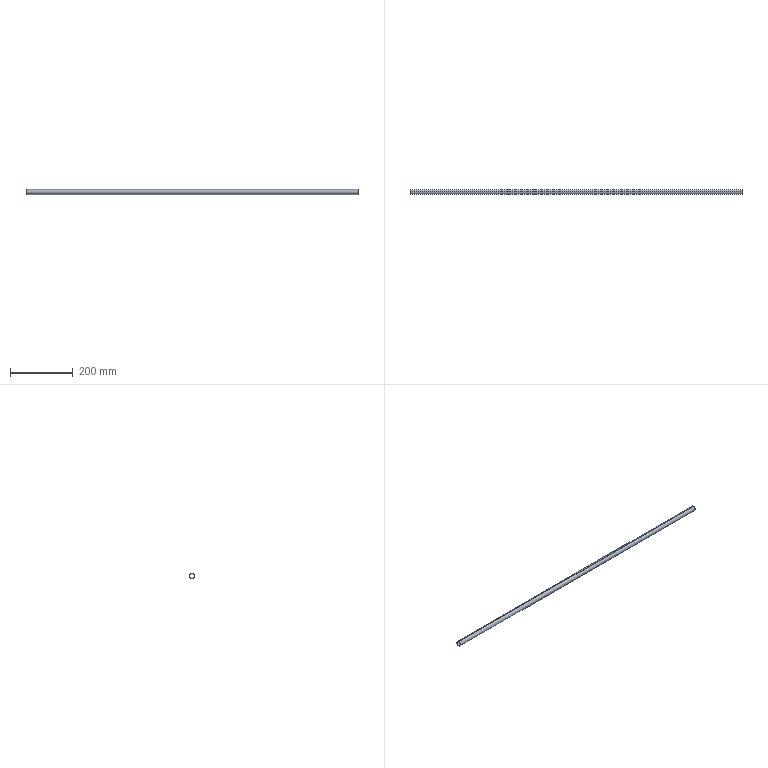Part | NX | features BREP 1 | 1 solid | 6 faces | box 1055 x 16 x 16 mm | volume 25686 mm3 | cylinder 4 | plane 2 | commonest cylinder face diameters 15 x2 16 x2
STEP:
#1=CARTESIAN_POINT('',(1055.,0.,7.5));
#2=VERTEX_POINT('',#1);
#3=CARTESIAN_POINT('',(1055.,0.,-7.5));
#4=VERTEX_POINT('',#3);
#5=CARTESIAN_POINT('',(1055.,0.,0.));
#6=DIRECTION('',(1.,0.,0.));
#7=DIRECTION('',(0.,0.,-1.));
#8=AXIS2_PLACEMENT_3D('',#5,#6,#7);
#9=CIRCLE('',#8,7.5);
#10=EDGE_CURVE('',#2,#4,#9,.T.);
#11=ORIENTED_EDGE('',*,*,#10,.T.);
#12=CARTESIAN_POINT('',(0.,0.,-7.5));
#13=VERTEX_POINT('',#12);
#14=CARTESIAN_POINT('',(1055.,0.,-7.5));
#15=DIRECTION('',(-1.,0.,0.));
#16=VECTOR('',#15,1000.);
#17=LINE('',#14,#16);
#18=EDGE_CURVE('',#4,#13,#17,.T.);
#19=ORIENTED_EDGE('',*,*,#18,.T.);
#20=CARTESIAN_POINT('',(0.,0.,7.5));
#21=VERTEX_POINT('',#20);
#22=CARTESIAN_POINT('',(0.,0.,0.));
#23=DIRECTION('',(1.,0.,0.));
#24=DIRECTION('',(0.,0.,-1.));
#25=AXIS2_PLACEMENT_3D('',#22,#23,#24);
#26=CIRCLE('',#25,7.5);
#27=EDGE_CURVE('',#21,#13,#26,.T.);
#28=ORIENTED_EDGE('',*,*,#27,.F.);
#29=CARTESIAN_POINT('',(1055.,0.,7.5));
#30=DIRECTION('',(-1.,0.,0.));
#31=VECTOR('',#30,1000.);
#32=LINE('',#29,#31);
#33=EDGE_CURVE('',#2,#21,#32,.T.);
#34=ORIENTED_EDGE('',*,*,#33,.F.);
#35=EDGE_LOOP('',(#11,#19,#28,#34));
#36=FACE_BOUND('',#35,.T.);
#37=CARTESIAN_POINT('',(1055.,0.,0.));
#38=DIRECTION('',(-1.,0.,0.));
#39=DIRECTION('',(0.,0.,-1.));
#40=AXIS2_PLACEMENT_3D('',#37,#38,#39);
#41=CYLINDRICAL_SURFACE('',#40,7.5);
#42=ADVANCED_FACE('',(#36),#41,.F.);
#43=CARTESIAN_POINT('',(1055.,0.,-8.));
#44=VERTEX_POINT('',#43);
#45=CARTESIAN_POINT('',(1055.,0.,8.));
#46=VERTEX_POINT('',#45);
#47=CARTESIAN_POINT('',(1055.,0.,0.));
#48=DIRECTION('',(1.,0.,0.));
#49=DIRECTION('',(0.,0.,-1.));
#50=AXIS2_PLACEMENT_3D('',#47,#48,#49);
#51=CIRCLE('',#50,8.);
#52=EDGE_CURVE('',#44,#46,#51,.T.);
#53=ORIENTED_EDGE('',*,*,#52,.F.);
#54=CARTESIAN_POINT('',(0.,0.,-8.));
#55=VERTEX_POINT('',#54);
#56=CARTESIAN_POINT('',(1055.,0.,-8.));
#57=DIRECTION('',(-1.,0.,0.));
#58=VECTOR('',#57,1000.);
#59=LINE('',#56,#58);
#60=EDGE_CURVE('',#44,#55,#59,.T.);
#61=ORIENTED_EDGE('',*,*,#60,.T.);
#62=CARTESIAN_POINT('',(0.,0.,8.));
#63=VERTEX_POINT('',#62);
#64=CARTESIAN_POINT('',(0.,0.,0.));
#65=DIRECTION('',(1.,0.,0.));
#66=DIRECTION('',(0.,0.,-1.));
#67=AXIS2_PLACEMENT_3D('',#64,#65,#66);
#68=CIRCLE('',#67,8.);
#69=EDGE_CURVE('',#55,#63,#68,.T.);
#70=ORIENTED_EDGE('',*,*,#69,.T.);
#71=CARTESIAN_POINT('',(1055.,0.,8.));
#72=DIRECTION('',(-1.,0.,0.));
#73=VECTOR('',#72,1000.);
#74=LINE('',#71,#73);
#75=EDGE_CURVE('',#46,#63,#74,.T.);
#76=ORIENTED_EDGE('',*,*,#75,.F.);
#77=EDGE_LOOP('',(#53,#61,#70,#76));
#78=FACE_BOUND('',#77,.T.);
#79=CARTESIAN_POINT('',(1055.,0.,0.));
#80=DIRECTION('',(-1.,0.,0.));
#81=DIRECTION('',(0.,0.,-1.));
#82=AXIS2_PLACEMENT_3D('',#79,#80,#81);
#83=CYLINDRICAL_SURFACE('',#82,8.);
#84=ADVANCED_FACE('',(#78),#83,.T.);
#85=CARTESIAN_POINT('',(1055.,0.,0.));
#86=DIRECTION('',(1.,0.,0.));
#87=DIRECTION('',(0.,0.,-1.));
#88=AXIS2_PLACEMENT_3D('',#85,#86,#87);
#89=CIRCLE('',#88,8.);
#90=EDGE_CURVE('',#46,#44,#89,.T.);
#91=ORIENTED_EDGE('',*,*,#90,.T.);
#92=ORIENTED_EDGE('',*,*,#52,.T.);
#93=EDGE_LOOP('',(#91,#92));
#94=FACE_BOUND('',#93,.T.);
#95=ORIENTED_EDGE('',*,*,#10,.F.);
#96=CARTESIAN_POINT('',(1055.,0.,0.));
#97=DIRECTION('',(1.,0.,0.));
#98=DIRECTION('',(0.,0.,-1.));
#99=AXIS2_PLACEMENT_3D('',#96,#97,#98);
#100=CIRCLE('',#99,7.5);
#101=EDGE_CURVE('',#4,#2,#100,.T.);
#102=ORIENTED_EDGE('',*,*,#101,.F.);
#103=EDGE_LOOP('',(#95,#102));
#104=FACE_BOUND('',#103,.T.);
#105=CARTESIAN_POINT('',(1055.,0.,0.));
#106=DIRECTION('',(1.,0.,0.));
#107=DIRECTION('',(0.,0.,-1.));
#108=AXIS2_PLACEMENT_3D('',#105,#106,#107);
#109=PLANE('',#108);
#110=ADVANCED_FACE('',(#94,#104),#109,.T.);
#111=CARTESIAN_POINT('',(0.,0.,0.));
#112=DIRECTION('',(1.,0.,0.));
#113=DIRECTION('',(0.,0.,-1.));
#114=AXIS2_PLACEMENT_3D('',#111,#112,#113);
#115=CIRCLE('',#114,8.);
#116=EDGE_CURVE('',#63,#55,#115,.T.);
#117=ORIENTED_EDGE('',*,*,#116,.F.);
#118=ORIENTED_EDGE('',*,*,#69,.F.);
#119=EDGE_LOOP('',(#117,#118));
#120=FACE_BOUND('',#119,.T.);
#121=ORIENTED_EDGE('',*,*,#27,.T.);
#122=CARTESIAN_POINT('',(0.,0.,0.));
#123=DIRECTION('',(1.,0.,0.));
#124=DIRECTION('',(0.,0.,-1.));
#125=AXIS2_PLACEMENT_3D('',#122,#123,#124);
#126=CIRCLE('',#125,7.5);
#127=EDGE_CURVE('',#13,#21,#126,.T.);
#128=ORIENTED_EDGE('',*,*,#127,.T.);
#129=EDGE_LOOP('',(#121,#128));
#130=FACE_BOUND('',#129,.T.);
#131=CARTESIAN_POINT('',(0.,0.,0.));
#132=DIRECTION('',(1.,0.,0.));
#133=DIRECTION('',(0.,0.,-1.));
#134=AXIS2_PLACEMENT_3D('',#131,#132,#133);
#135=PLANE('',#134);
#136=ADVANCED_FACE('',(#120,#130),#135,.F.);
#137=ORIENTED_EDGE('',*,*,#60,.F.);
#138=ORIENTED_EDGE('',*,*,#90,.F.);
#139=ORIENTED_EDGE('',*,*,#75,.T.);
#140=ORIENTED_EDGE('',*,*,#116,.T.);
#141=EDGE_LOOP('',(#137,#138,#139,#140));
#142=FACE_BOUND('',#141,.T.);
#143=CARTESIAN_POINT('',(1055.,0.,0.));
#144=DIRECTION('',(-1.,0.,0.));
#145=DIRECTION('',(0.,0.,-1.));
#146=AXIS2_PLACEMENT_3D('',#143,#144,#145);
#147=CYLINDRICAL_SURFACE('',#146,8.);
#148=ADVANCED_FACE('',(#142),#147,.T.);
#149=ORIENTED_EDGE('',*,*,#18,.F.);
#150=ORIENTED_EDGE('',*,*,#101,.T.);
#151=ORIENTED_EDGE('',*,*,#33,.T.);
#152=ORIENTED_EDGE('',*,*,#127,.F.);
#153=EDGE_LOOP('',(#149,#150,#151,#152));
#154=FACE_BOUND('',#153,.T.);
#155=CARTESIAN_POINT('',(1055.,0.,0.));
#156=DIRECTION('',(-1.,0.,0.));
#157=DIRECTION('',(0.,0.,-1.));
#158=AXIS2_PLACEMENT_3D('',#155,#156,#157);
#159=CYLINDRICAL_SURFACE('',#158,7.5);
#160=ADVANCED_FACE('',(#154),#159,.F.);
#161=CLOSED_SHELL('',(#42,#84,#110,#136,#148,#160));
#162=MANIFOLD_SOLID_BREP('',#161);
#163=(LENGTH_UNIT()NAMED_UNIT(*)SI_UNIT(.MILLI.,.METRE.));
#164=UNCERTAINTY_MEASURE_WITH_UNIT(LENGTH_MEASURE(0.00001),#163,'','');
#165=(NAMED_UNIT(*)PLANE_ANGLE_UNIT()SI_UNIT($,.RADIAN.));
#166=(NAMED_UNIT(*)SI_UNIT($,.STERADIAN.)SOLID_ANGLE_UNIT());
#167=(GEOMETRIC_REPRESENTATION_CONTEXT(3)GLOBAL_UNCERTAINTY_ASSIGNED_CONTEXT((#164))GLOBAL_UNIT_ASSIGNED_CONTEXT((#163,#165,#166))REPRESENTATION_CONTEXT('',''));
#168=ADVANCED_BREP_SHAPE_REPRESENTATION('',(#162),#167);